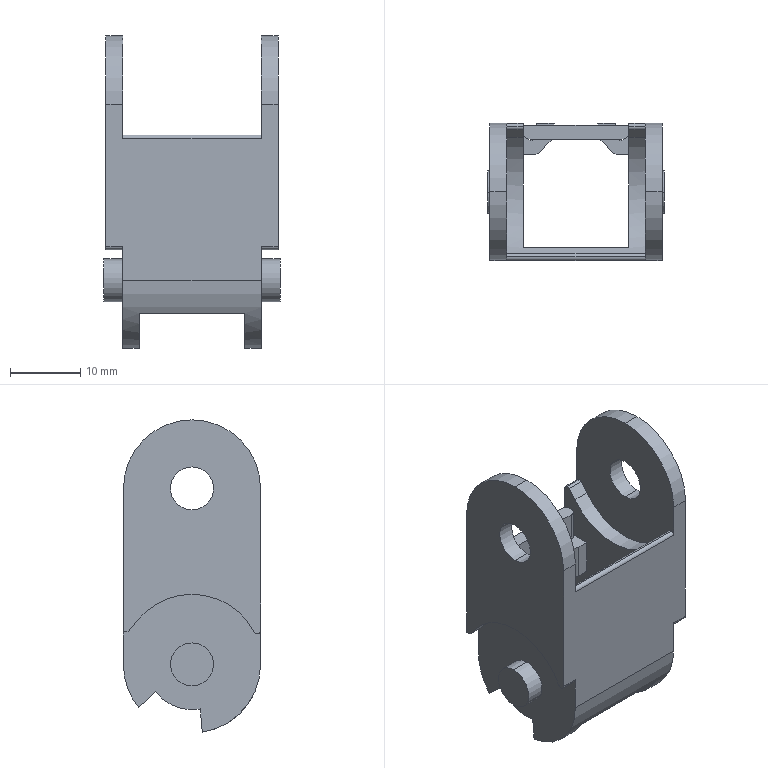Part | STEP file | _VBD02-F15-R28-N20-001.stp | 1 solid | 89 faces | box 25.1 x 19.5 x 44.39 mm | volume 5553 mm3 | plane 47 | cylinder 42 | commonest cylinder face diameters 1 x10 6.1 x8 19.5 x7 2 x6 19.9 x5 2.4 x4